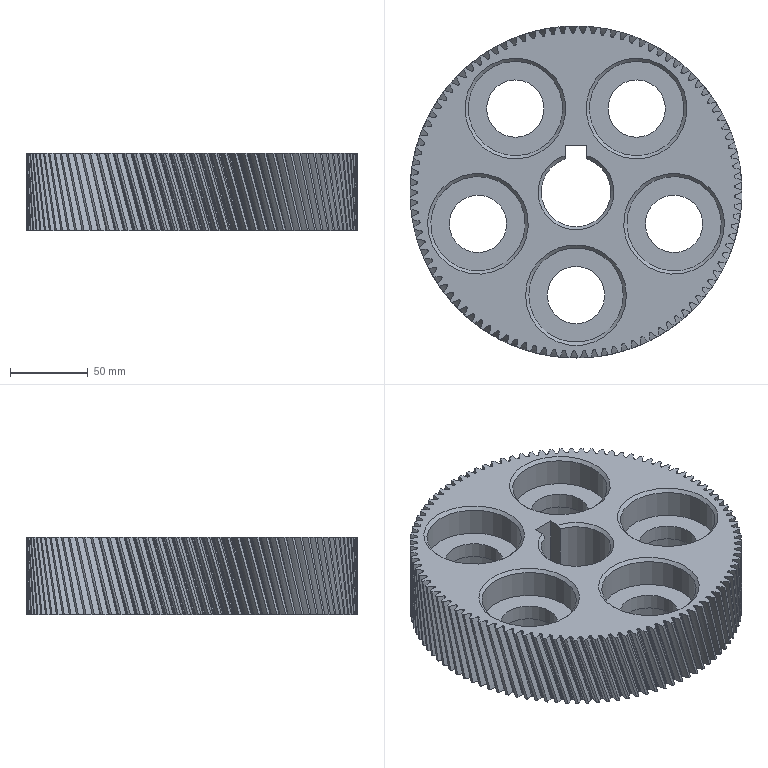Part | NX | 1 solid | 649 faces | box 214.08 x 214.08 x 50 mm | volume 1001272 mm3 | spline 505 | cylinder 117 | plane 15 | cone 12 | commonest cylinder face diameters 205.08 x101 61 x10 37 x5 45 x1